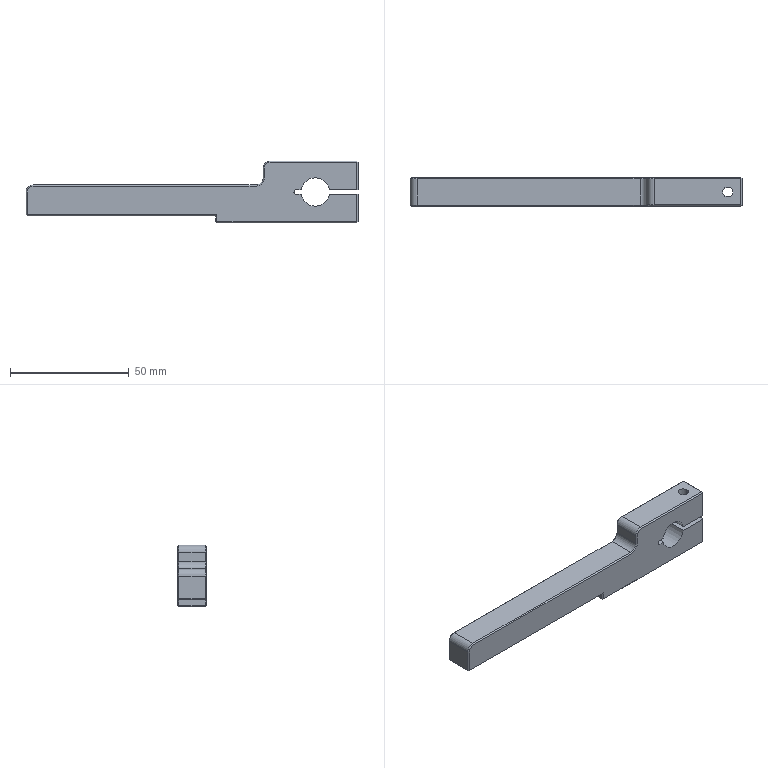Part | STEP file | ND25021-01-JDKM-66-TL | 1 solid | 71 faces | box 140 x 12 x 26 mm | volume 26347 mm3 | plane 45 | cylinder 16 | cone 10 | commonest cylinder face diameters 3.3 x4 6 x3 12 x3 2 x2 4.2 x2 5.5 x2